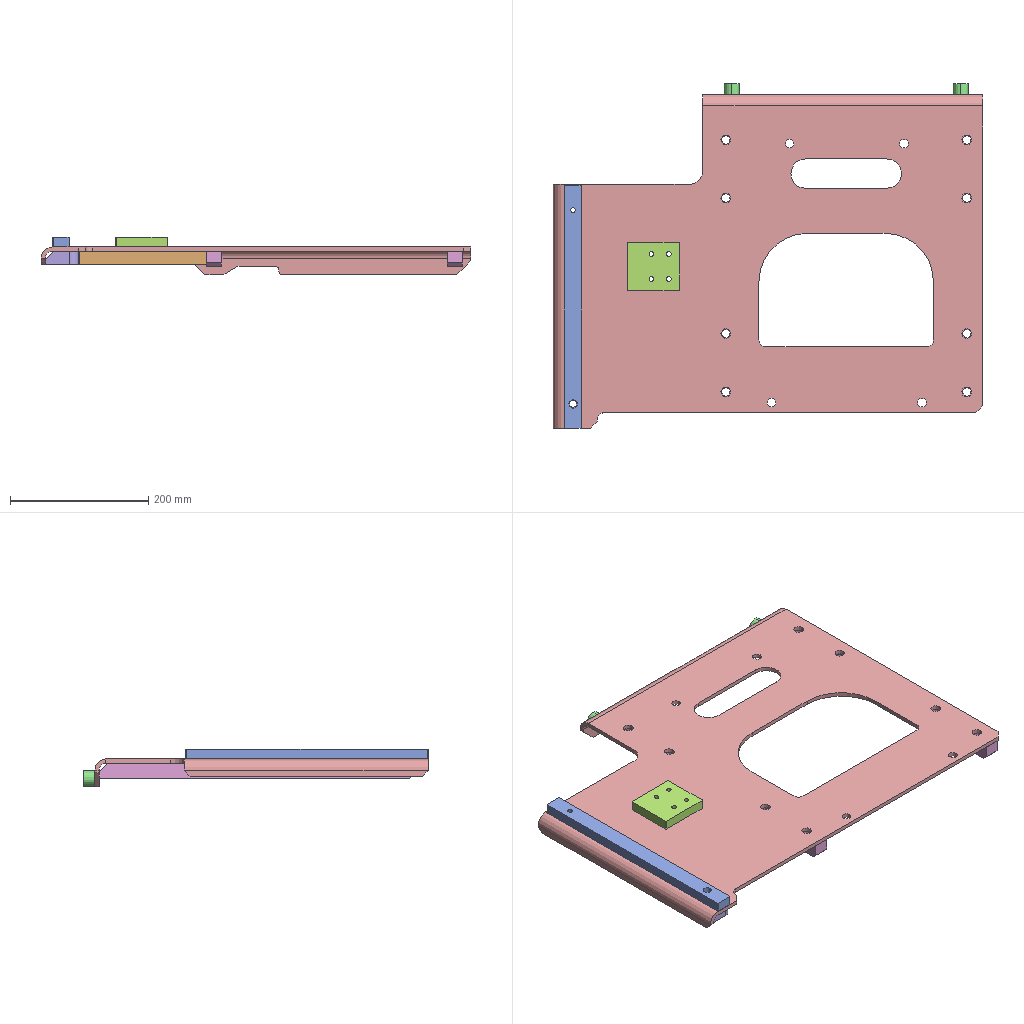Assembly | SolidWorks | 8 different items | 12 placed | box 620 x 497 x 54 mm
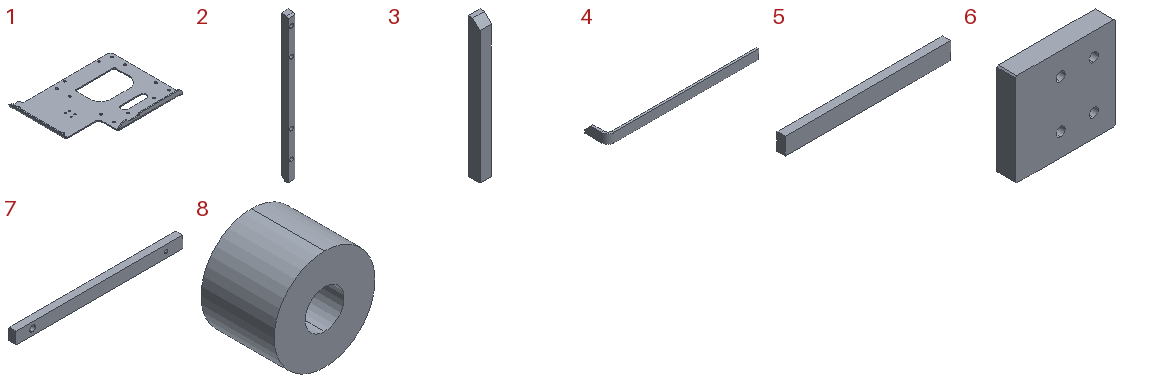Parts list (item | quantity | size | volume | features):
1 | x1 | 620 x 481.4 x 40 mm | 1351039 mm3 | features ICE 7, Chamfer 3, EdgeFlange 2, Fillet 2, SMBaseFlange 2, FlatPattern 1, SheetMetal 1
2 | x2 | 22 x 22 x 453 mm | 207440 mm3 | features Chamfer 2, Extrusion 1, ICE 1
3 | x1 | 19 x 19 x 231.5 mm | 82203 mm3 | features Chamfer 1, Extrusion 1
4 | x1 | 313 x 47.5 x 19 mm | 29738 mm3 | features Chamfer 1, FlatPattern 1, SMBaseFlange 1, SheetMetal 1
5 | x2 | 183.5 x 9 x 19 mm | 31378 mm3 | features FlatPattern 1, SMBaseFlange 1, SheetMetal 1
6 | x1 | 75 x 14 x 70 mm | 71438 mm3 | features FlatPattern 1, HoleWzd 1, SMBaseFlange 1, SheetMetal 1
7 | x1 | 350 x 14 x 25 mm | 120380 mm3 | features FlatPattern 1, HoleWzd 1, SMBaseFlange 1, SheetMetal 1
8 | x3 | 22 x 16 x 22 mm | 5174 mm3 | features Extrusion 1, HoleWzd 1
Mates (type | each side: item.copy, entity, surface, feature):
Coincident | 1.1 face plane Base-Flange1 | 7.1 face plane Base-Flange1
Concentric | 1.1 face cylinder Cut-Extrude6 | 7.1 face cylinder Base-Flange1
Concentric | 1.1 face cylinder Cut-Extrude6 | 7.1 edge
Coincident | 1.1 face plane Base-Flange1 | 6.1 face plane Base-Flange1
Concentric | 1.1 face cylinder Cut-Extrude6 | 6.1 face cylinder M8 Tapped Hole1 | 2 times
Coincident | 1.1 face plane Base-Flange1 | 2.1 face plane Boss-Extrude1
Concentric | 1.1 face cylinder Cut-Extrude3 | 2.1 face cylinder Cut-Extrude1 | 2 times
Coincident | 1.1 face plane Base-Flange1 | 2.2 face plane Boss-Extrude1
Concentric | 1.1 face cylinder Cut-Extrude3 | 2.2 face cylinder Cut-Extrude1 | 2 times
Coincident | 1.1 face plane Base-Flange1 | 3.1 face plane Boss-Extrude1
DistanceDim | 1.1 face plane Cut-Extrude1 | 3.1 face plane Boss-Extrude1
Coincident | 2.2 face plane Boss-Extrude1 | 3.1 face plane Boss-Extrude1
DistanceDim | 3.1 face plane Boss-Extrude1 | 5.1 face plane Base-Flange1
Coincident | 2.2 face plane Boss-Extrude1 | 5.1 face plane Base-Flange1
Coincident | 1.1 face plane Base-Flange1 | 5.1 edge
Coincident | 1.1 face plane Base-Flange1 | 4.1 edge
Coincident | 3.1 face plane Boss-Extrude1 | 4.1 face plane Base-Flange1
Coincident | 1.1 face plane Edge-Flange1 | 4.1 face plane Base-Flange1
Coincident | 1.1 face plane Edge-Flange3 | 8.1 face plane Boss-Extrude1
DistanceDim | 1.1 face plane Base-Flange1 | 8.1 face cylinder Boss-Extrude1
DistanceDim | 8.1 face cylinder Boss-Extrude1 | 1.1 face plane Base-Flange1
Coincident | 1.1 face plane Base-Flange1 | 8.2 edge
DistanceDim | 8.2 face cylinder M10 Tapped Hole1 | 1.1 face plane Cut-Extrude1
DistanceDim | 8.2 face cylinder M10 Tapped Hole1 | 1.1 face plane Edge-Flange1